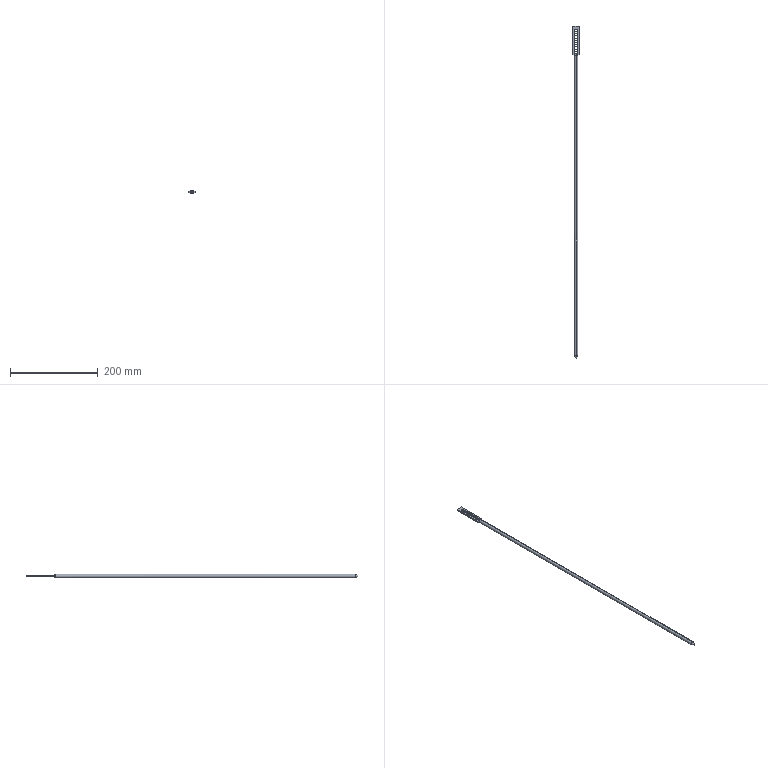Part | SolidWorks | 1 solid | 49 faces | box 14 x 756 x 8 mm | volume 36761 mm3 | cylinder 35 | plane 8 | torus 4 | cone 2 | commonest cylinder face diameters 6.1 x33 8 x2